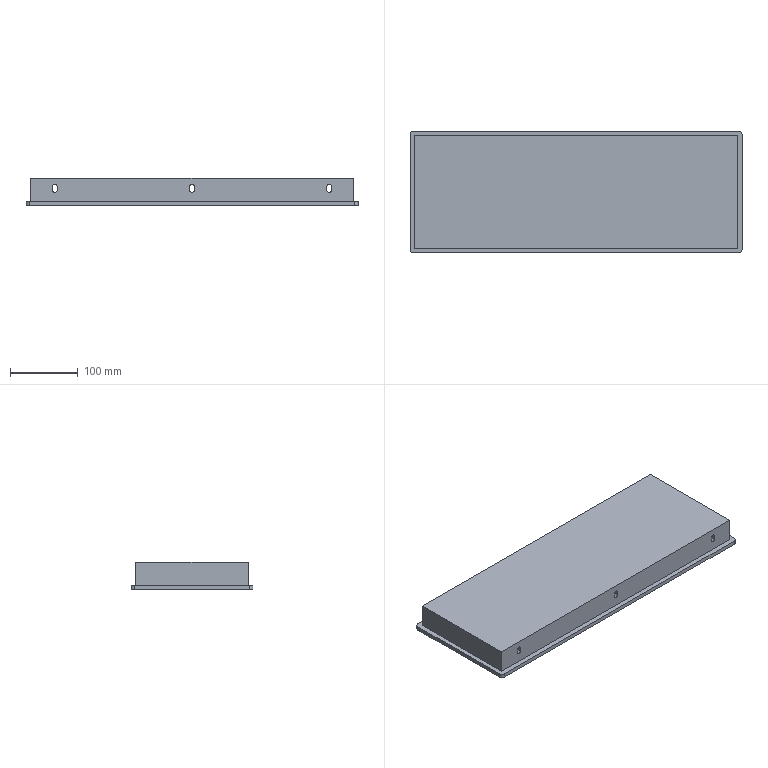Part | 1 solid | 30 faces | box 490 x 180 x 41 mm | volume 3258036 mm3 | plane 17 | cylinder 13 | commonest cylinder face diameters 7 x9 10 x4
STEP:
#1=CARTESIAN_POINT('',(-202.5,-83.,32.));
#2=VERTEX_POINT('',#1);
#3=CARTESIAN_POINT('',(-199.,-83.,28.5));
#4=VERTEX_POINT('',#3);
#5=CARTESIAN_POINT('',(-202.5,-83.,28.5));
#6=DIRECTION('',(0.,1.,0.));
#7=DIRECTION('',(0.,0.,1.));
#8=AXIS2_PLACEMENT_3D('',#5,#6,#7);
#9=CIRCLE('',#8,3.5);
#10=EDGE_CURVE('',#2,#4,#9,.T.);
#11=ORIENTED_EDGE('',*,*,#10,.F.);
#12=CARTESIAN_POINT('',(-202.5,83.,32.));
#13=VERTEX_POINT('',#12);
#14=CARTESIAN_POINT('',(-202.5,-90.,32.));
#15=DIRECTION('',(0.,1.,0.));
#16=VECTOR('',#15,1000.);
#17=LINE('',#14,#16);
#18=EDGE_CURVE('',#2,#13,#17,.T.);
#19=ORIENTED_EDGE('',*,*,#18,.T.);
#20=CARTESIAN_POINT('',(-199.,83.,28.5));
#21=VERTEX_POINT('',#20);
#22=CARTESIAN_POINT('',(-202.5,83.,28.5));
#23=DIRECTION('',(0.,-1.,0.));
#24=DIRECTION('',(0.,0.,-1.));
#25=AXIS2_PLACEMENT_3D('',#22,#23,#24);
#26=CIRCLE('',#25,3.5);
#27=EDGE_CURVE('',#21,#13,#26,.T.);
#28=ORIENTED_EDGE('',*,*,#27,.F.);
#29=CARTESIAN_POINT('',(-199.,-90.,28.5));
#30=DIRECTION('',(0.,1.,0.));
#31=VECTOR('',#30,1000.);
#32=LINE('',#29,#31);
#33=EDGE_CURVE('',#4,#21,#32,.T.);
#34=ORIENTED_EDGE('',*,*,#33,.F.);
#35=EDGE_LOOP('',(#11,#19,#28,#34));
#36=FACE_OUTER_BOUND('',#35,.T.);
#37=CARTESIAN_POINT('',(-202.5,-90.,28.5));
#38=DIRECTION('',(0.,1.,0.));
#39=DIRECTION('',(0.,0.,1.));
#40=AXIS2_PLACEMENT_3D('',#37,#38,#39);
#41=CYLINDRICAL_SURFACE('',#40,3.5);
#42=ADVANCED_FACE('',(#36),#41,.F.);
#43=CARTESIAN_POINT('',(0.,-83.,32.));
#44=VERTEX_POINT('',#43);
#45=CARTESIAN_POINT('',(3.5,-83.,28.5));
#46=VERTEX_POINT('',#45);
#47=CARTESIAN_POINT('',(0.,-83.,28.5));
#48=DIRECTION('',(0.,1.,0.));
#49=DIRECTION('',(0.,0.,1.));
#50=AXIS2_PLACEMENT_3D('',#47,#48,#49);
#51=CIRCLE('',#50,3.5);
#52=EDGE_CURVE('',#44,#46,#51,.T.);
#53=ORIENTED_EDGE('',*,*,#52,.F.);
#54=CARTESIAN_POINT('',(0.,83.,32.));
#55=VERTEX_POINT('',#54);
#56=CARTESIAN_POINT('',(0.,-90.,32.));
#57=DIRECTION('',(0.,1.,0.));
#58=VECTOR('',#57,1000.);
#59=LINE('',#56,#58);
#60=EDGE_CURVE('',#44,#55,#59,.T.);
#61=ORIENTED_EDGE('',*,*,#60,.T.);
#62=CARTESIAN_POINT('',(3.5,83.,28.5));
#63=VERTEX_POINT('',#62);
#64=CARTESIAN_POINT('',(0.,83.,28.5));
#65=DIRECTION('',(0.,-1.,0.));
#66=DIRECTION('',(0.,0.,-1.));
#67=AXIS2_PLACEMENT_3D('',#64,#65,#66);
#68=CIRCLE('',#67,3.5);
#69=EDGE_CURVE('',#63,#55,#68,.T.);
#70=ORIENTED_EDGE('',*,*,#69,.F.);
#71=CARTESIAN_POINT('',(3.5,-90.,28.5));
#72=DIRECTION('',(0.,1.,0.));
#73=VECTOR('',#72,1000.);
#74=LINE('',#71,#73);
#75=EDGE_CURVE('',#46,#63,#74,.T.);
#76=ORIENTED_EDGE('',*,*,#75,.F.);
#77=EDGE_LOOP('',(#53,#61,#70,#76));
#78=FACE_OUTER_BOUND('',#77,.T.);
#79=CARTESIAN_POINT('',(0.,-90.,28.5));
#80=DIRECTION('',(0.,1.,0.));
#81=DIRECTION('',(0.,0.,1.));
#82=AXIS2_PLACEMENT_3D('',#79,#80,#81);
#83=CYLINDRICAL_SURFACE('',#82,3.5);
#84=ADVANCED_FACE('',(#78),#83,.F.);
#85=CARTESIAN_POINT('',(202.5,-83.,32.));
#86=VERTEX_POINT('',#85);
#87=CARTESIAN_POINT('',(206.,-83.,28.5));
#88=VERTEX_POINT('',#87);
#89=CARTESIAN_POINT('',(202.5,-83.,28.5));
#90=DIRECTION('',(0.,1.,0.));
#91=DIRECTION('',(0.,0.,1.));
#92=AXIS2_PLACEMENT_3D('',#89,#90,#91);
#93=CIRCLE('',#92,3.5);
#94=EDGE_CURVE('',#86,#88,#93,.T.);
#95=ORIENTED_EDGE('',*,*,#94,.F.);
#96=CARTESIAN_POINT('',(202.5,83.,32.));
#97=VERTEX_POINT('',#96);
#98=CARTESIAN_POINT('',(202.5,-90.,32.));
#99=DIRECTION('',(0.,1.,0.));
#100=VECTOR('',#99,1000.);
#101=LINE('',#98,#100);
#102=EDGE_CURVE('',#86,#97,#101,.T.);
#103=ORIENTED_EDGE('',*,*,#102,.T.);
#104=CARTESIAN_POINT('',(206.,83.,28.5));
#105=VERTEX_POINT('',#104);
#106=CARTESIAN_POINT('',(202.5,83.,28.5));
#107=DIRECTION('',(0.,-1.,0.));
#108=DIRECTION('',(0.,0.,-1.));
#109=AXIS2_PLACEMENT_3D('',#106,#107,#108);
#110=CIRCLE('',#109,3.5);
#111=EDGE_CURVE('',#105,#97,#110,.T.);
#112=ORIENTED_EDGE('',*,*,#111,.F.);
#113=CARTESIAN_POINT('',(206.,-90.,28.5));
#114=DIRECTION('',(0.,1.,0.));
#115=VECTOR('',#114,1000.);
#116=LINE('',#113,#115);
#117=EDGE_CURVE('',#88,#105,#116,.T.);
#118=ORIENTED_EDGE('',*,*,#117,.F.);
#119=EDGE_LOOP('',(#95,#103,#112,#118));
#120=FACE_OUTER_BOUND('',#119,.T.);
#121=CARTESIAN_POINT('',(202.5,-90.,28.5));
#122=DIRECTION('',(0.,1.,0.));
#123=DIRECTION('',(0.,0.,1.));
#124=AXIS2_PLACEMENT_3D('',#121,#122,#123);
#125=CYLINDRICAL_SURFACE('',#124,3.5);
#126=ADVANCED_FACE('',(#120),#125,.F.);
#127=CARTESIAN_POINT('',(245.,-85.,0.));
#128=VERTEX_POINT('',#127);
#129=CARTESIAN_POINT('',(245.,85.,0.));
#130=VERTEX_POINT('',#129);
#131=CARTESIAN_POINT('',(245.,90.,0.));
#132=DIRECTION('',(0.,1.,0.));
#133=VECTOR('',#132,1000.);
#134=LINE('',#131,#133);
#135=EDGE_CURVE('',#128,#130,#134,.T.);
#136=ORIENTED_EDGE('',*,*,#135,.T.);
#137=CARTESIAN_POINT('',(245.,85.,6.));
#138=VERTEX_POINT('',#137);
#139=CARTESIAN_POINT('',(245.,85.,6.));
#140=DIRECTION('',(0.,0.,1.));
#141=VECTOR('',#140,1000.);
#142=LINE('',#139,#141);
#143=EDGE_CURVE('',#130,#138,#142,.T.);
#144=ORIENTED_EDGE('',*,*,#143,.T.);
#145=CARTESIAN_POINT('',(245.,-85.,6.));
#146=VERTEX_POINT('',#145);
#147=CARTESIAN_POINT('',(245.,90.,6.));
#148=DIRECTION('',(0.,1.,0.));
#149=VECTOR('',#148,1000.);
#150=LINE('',#147,#149);
#151=EDGE_CURVE('',#146,#138,#150,.T.);
#152=ORIENTED_EDGE('',*,*,#151,.F.);
#153=CARTESIAN_POINT('',(245.,-85.,6.));
#154=DIRECTION('',(0.,0.,-1.));
#155=VECTOR('',#154,1000.);
#156=LINE('',#153,#155);
#157=EDGE_CURVE('',#146,#128,#156,.T.);
#158=ORIENTED_EDGE('',*,*,#157,.T.);
#159=EDGE_LOOP('',(#136,#144,#152,#158));
#160=FACE_OUTER_BOUND('',#159,.T.);
#161=CARTESIAN_POINT('',(245.,90.,6.));
#162=DIRECTION('',(-1.,0.,0.));
#163=DIRECTION('',(0.,0.,1.));
#164=AXIS2_PLACEMENT_3D('',#161,#162,#163);
#165=PLANE('',#164);
#166=ADVANCED_FACE('',(#160),#165,.F.);
#167=CARTESIAN_POINT('',(240.,90.,6.));
#168=VERTEX_POINT('',#167);
#169=CARTESIAN_POINT('',(-240.,90.,6.));
#170=VERTEX_POINT('',#169);
#171=CARTESIAN_POINT('',(-245.,90.,6.));
#172=DIRECTION('',(-1.,0.,0.));
#173=VECTOR('',#172,1000.);
#174=LINE('',#171,#173);
#175=EDGE_CURVE('',#168,#170,#174,.T.);
#176=ORIENTED_EDGE('',*,*,#175,.F.);
#177=CARTESIAN_POINT('',(240.,90.,0.));
#178=VERTEX_POINT('',#177);
#179=CARTESIAN_POINT('',(240.,90.,6.));
#180=DIRECTION('',(0.,0.,-1.));
#181=VECTOR('',#180,1000.);
#182=LINE('',#179,#181);
#183=EDGE_CURVE('',#168,#178,#182,.T.);
#184=ORIENTED_EDGE('',*,*,#183,.T.);
#185=CARTESIAN_POINT('',(-240.,90.,0.));
#186=VERTEX_POINT('',#185);
#187=CARTESIAN_POINT('',(-245.,90.,0.));
#188=DIRECTION('',(-1.,0.,0.));
#189=VECTOR('',#188,1000.);
#190=LINE('',#187,#189);
#191=EDGE_CURVE('',#178,#186,#190,.T.);
#192=ORIENTED_EDGE('',*,*,#191,.T.);
#193=CARTESIAN_POINT('',(-240.,90.,6.));
#194=DIRECTION('',(0.,0.,1.));
#195=VECTOR('',#194,1000.);
#196=LINE('',#193,#195);
#197=EDGE_CURVE('',#186,#170,#196,.T.);
#198=ORIENTED_EDGE('',*,*,#197,.T.);
#199=EDGE_LOOP('',(#176,#184,#192,#198));
#200=FACE_OUTER_BOUND('',#199,.T.);
#201=CARTESIAN_POINT('',(-245.,90.,6.));
#202=DIRECTION('',(0.,-1.,0.));
#203=DIRECTION('',(0.,0.,-1.));
#204=AXIS2_PLACEMENT_3D('',#201,#202,#203);
#205=PLANE('',#204);
#206=ADVANCED_FACE('',(#200),#205,.F.);
#207=CARTESIAN_POINT('',(-245.,85.,0.));
#208=VERTEX_POINT('',#207);
#209=CARTESIAN_POINT('',(-245.,-85.,0.));
#210=VERTEX_POINT('',#209);
#211=CARTESIAN_POINT('',(-245.,90.,0.));
#212=DIRECTION('',(0.,-1.,0.));
#213=VECTOR('',#212,1000.);
#214=LINE('',#211,#213);
#215=EDGE_CURVE('',#208,#210,#214,.T.);
#216=ORIENTED_EDGE('',*,*,#215,.T.);
#217=CARTESIAN_POINT('',(-245.,-85.,6.));
#218=VERTEX_POINT('',#217);
#219=CARTESIAN_POINT('',(-245.,-85.,6.));
#220=DIRECTION('',(0.,0.,1.));
#221=VECTOR('',#220,1000.);
#222=LINE('',#219,#221);
#223=EDGE_CURVE('',#210,#218,#222,.T.);
#224=ORIENTED_EDGE('',*,*,#223,.T.);
#225=CARTESIAN_POINT('',(-245.,85.,6.));
#226=VERTEX_POINT('',#225);
#227=CARTESIAN_POINT('',(-245.,90.,6.));
#228=DIRECTION('',(0.,-1.,0.));
#229=VECTOR('',#228,1000.);
#230=LINE('',#227,#229);
#231=EDGE_CURVE('',#226,#218,#230,.T.);
#232=ORIENTED_EDGE('',*,*,#231,.F.);
#233=CARTESIAN_POINT('',(-245.,85.,6.));
#234=DIRECTION('',(0.,0.,-1.));
#235=VECTOR('',#234,1000.);
#236=LINE('',#233,#235);
#237=EDGE_CURVE('',#226,#208,#236,.T.);
#238=ORIENTED_EDGE('',*,*,#237,.T.);
#239=EDGE_LOOP('',(#216,#224,#232,#238));
#240=FACE_OUTER_BOUND('',#239,.T.);
#241=CARTESIAN_POINT('',(-245.,90.,6.));
#242=DIRECTION('',(1.,0.,0.));
#243=DIRECTION('',(0.,0.,-1.));
#244=AXIS2_PLACEMENT_3D('',#241,#242,#243);
#245=PLANE('',#244);
#246=ADVANCED_FACE('',(#240),#245,.F.);
#247=CARTESIAN_POINT('',(-240.,-90.,0.));
#248=VERTEX_POINT('',#247);
#249=CARTESIAN_POINT('',(240.,-90.,0.));
#250=VERTEX_POINT('',#249);
#251=CARTESIAN_POINT('',(-245.,-90.,0.));
#252=DIRECTION('',(1.,0.,0.));
#253=VECTOR('',#252,1000.);
#254=LINE('',#251,#253);
#255=EDGE_CURVE('',#248,#250,#254,.T.);
#256=ORIENTED_EDGE('',*,*,#255,.T.);
#257=CARTESIAN_POINT('',(240.,-90.,6.));
#258=VERTEX_POINT('',#257);
#259=CARTESIAN_POINT('',(240.,-90.,6.));
#260=DIRECTION('',(0.,0.,1.));
#261=VECTOR('',#260,1000.);
#262=LINE('',#259,#261);
#263=EDGE_CURVE('',#250,#258,#262,.T.);
#264=ORIENTED_EDGE('',*,*,#263,.T.);
#265=CARTESIAN_POINT('',(-240.,-90.,6.));
#266=VERTEX_POINT('',#265);
#267=CARTESIAN_POINT('',(-245.,-90.,6.));
#268=DIRECTION('',(1.,0.,0.));
#269=VECTOR('',#268,1000.);
#270=LINE('',#267,#269);
#271=EDGE_CURVE('',#266,#258,#270,.T.);
#272=ORIENTED_EDGE('',*,*,#271,.F.);
#273=CARTESIAN_POINT('',(-240.,-90.,6.));
#274=DIRECTION('',(0.,0.,-1.));
#275=VECTOR('',#274,1000.);
#276=LINE('',#273,#275);
#277=EDGE_CURVE('',#266,#248,#276,.T.);
#278=ORIENTED_EDGE('',*,*,#277,.T.);
#279=EDGE_LOOP('',(#256,#264,#272,#278));
#280=FACE_OUTER_BOUND('',#279,.T.);
#281=CARTESIAN_POINT('',(-245.,-90.,6.));
#282=DIRECTION('',(0.,1.,0.));
#283=DIRECTION('',(0.,0.,1.));
#284=AXIS2_PLACEMENT_3D('',#281,#282,#283);
#285=PLANE('',#284);
#286=ADVANCED_FACE('',(#280),#285,.F.);
#287=CARTESIAN_POINT('',(238.,-83.,6.));
#288=VERTEX_POINT('',#287);
#289=CARTESIAN_POINT('',(238.,83.,6.));
#290=VERTEX_POINT('',#289);
#291=CARTESIAN_POINT('',(238.,83.,6.));
#292=DIRECTION('',(0.,1.,0.));
#293=VECTOR('',#292,1000.);
#294=LINE('',#291,#293);
#295=EDGE_CURVE('',#288,#290,#294,.T.);
#296=ORIENTED_EDGE('',*,*,#295,.F.);
#297=CARTESIAN_POINT('',(-238.,-83.,6.));
#298=VERTEX_POINT('',#297);
#299=CARTESIAN_POINT('',(-238.,-83.,6.));
#300=DIRECTION('',(1.,0.,0.));
#301=VECTOR('',#300,1000.);
#302=LINE('',#299,#301);
#303=EDGE_CURVE('',#298,#288,#302,.T.);
#304=ORIENTED_EDGE('',*,*,#303,.F.);
#305=CARTESIAN_POINT('',(-238.,83.,6.));
#306=VERTEX_POINT('',#305);
#307=CARTESIAN_POINT('',(-238.,83.,6.));
#308=DIRECTION('',(0.,-1.,0.));
#309=VECTOR('',#308,1000.);
#310=LINE('',#307,#309);
#311=EDGE_CURVE('',#306,#298,#310,.T.);
#312=ORIENTED_EDGE('',*,*,#311,.F.);
#313=CARTESIAN_POINT('',(-238.,83.,6.));
#314=DIRECTION('',(-1.,0.,0.));
#315=VECTOR('',#314,1000.);
#316=LINE('',#313,#315);
#317=EDGE_CURVE('',#290,#306,#316,.T.);
#318=ORIENTED_EDGE('',*,*,#317,.F.);
#319=EDGE_LOOP('',(#296,#304,#312,#318));
#320=FACE_BOUND('',#319,.T.);
#321=ORIENTED_EDGE('',*,*,#151,.T.);
#322=CARTESIAN_POINT('',(240.,85.,6.));
#323=DIRECTION('',(0.,0.,1.));
#324=DIRECTION('',(1.,0.,0.));
#325=AXIS2_PLACEMENT_3D('',#322,#323,#324);
#326=CIRCLE('',#325,5.);
#327=EDGE_CURVE('',#138,#168,#326,.T.);
#328=ORIENTED_EDGE('',*,*,#327,.T.);
#329=ORIENTED_EDGE('',*,*,#175,.T.);
#330=CARTESIAN_POINT('',(-240.,85.,6.));
#331=DIRECTION('',(0.,0.,1.));
#332=DIRECTION('',(1.,0.,0.));
#333=AXIS2_PLACEMENT_3D('',#330,#331,#332);
#334=CIRCLE('',#333,5.);
#335=EDGE_CURVE('',#170,#226,#334,.T.);
#336=ORIENTED_EDGE('',*,*,#335,.T.);
#337=ORIENTED_EDGE('',*,*,#231,.T.);
#338=CARTESIAN_POINT('',(-240.,-85.,6.));
#339=DIRECTION('',(0.,0.,1.));
#340=DIRECTION('',(1.,0.,0.));
#341=AXIS2_PLACEMENT_3D('',#338,#339,#340);
#342=CIRCLE('',#341,5.);
#343=EDGE_CURVE('',#218,#266,#342,.T.);
#344=ORIENTED_EDGE('',*,*,#343,.T.);
#345=ORIENTED_EDGE('',*,*,#271,.T.);
#346=CARTESIAN_POINT('',(240.,-85.,6.));
#347=DIRECTION('',(0.,0.,1.));
#348=DIRECTION('',(1.,0.,0.));
#349=AXIS2_PLACEMENT_3D('',#346,#347,#348);
#350=CIRCLE('',#349,5.);
#351=EDGE_CURVE('',#258,#146,#350,.T.);
#352=ORIENTED_EDGE('',*,*,#351,.T.);
#353=EDGE_LOOP('',(#321,#328,#329,#336,#337,#344,#345,#352));
#354=FACE_OUTER_BOUND('',#353,.T.);
#355=CARTESIAN_POINT('',(0.,0.,6.));
#356=DIRECTION('',(0.,0.,1.));
#357=DIRECTION('',(1.,0.,0.));
#358=AXIS2_PLACEMENT_3D('',#355,#356,#357);
#359=PLANE('',#358);
#360=ADVANCED_FACE('',(#320,#354),#359,.T.);
#361=ORIENTED_EDGE('',*,*,#191,.F.);
#362=CARTESIAN_POINT('',(240.,85.,0.));
#363=DIRECTION('',(0.,0.,-1.));
#364=DIRECTION('',(1.,0.,0.));
#365=AXIS2_PLACEMENT_3D('',#362,#363,#364);
#366=CIRCLE('',#365,5.);
#367=EDGE_CURVE('',#178,#130,#366,.T.);
#368=ORIENTED_EDGE('',*,*,#367,.T.);
#369=ORIENTED_EDGE('',*,*,#135,.F.);
#370=CARTESIAN_POINT('',(240.,-85.,0.));
#371=DIRECTION('',(0.,0.,-1.));
#372=DIRECTION('',(1.,0.,0.));
#373=AXIS2_PLACEMENT_3D('',#370,#371,#372);
#374=CIRCLE('',#373,5.);
#375=EDGE_CURVE('',#128,#250,#374,.T.);
#376=ORIENTED_EDGE('',*,*,#375,.T.);
#377=ORIENTED_EDGE('',*,*,#255,.F.);
#378=CARTESIAN_POINT('',(-240.,-85.,0.));
#379=DIRECTION('',(0.,0.,-1.));
#380=DIRECTION('',(1.,0.,0.));
#381=AXIS2_PLACEMENT_3D('',#378,#379,#380);
#382=CIRCLE('',#381,5.);
#383=EDGE_CURVE('',#248,#210,#382,.T.);
#384=ORIENTED_EDGE('',*,*,#383,.T.);
#385=ORIENTED_EDGE('',*,*,#215,.F.);
#386=CARTESIAN_POINT('',(-240.,85.,0.));
#387=DIRECTION('',(0.,0.,-1.));
#388=DIRECTION('',(1.,0.,0.));
#389=AXIS2_PLACEMENT_3D('',#386,#387,#388);
#390=CIRCLE('',#389,5.);
#391=EDGE_CURVE('',#208,#186,#390,.T.);
#392=ORIENTED_EDGE('',*,*,#391,.T.);
#393=EDGE_LOOP('',(#361,#368,#369,#376,#377,#384,#385,#392));
#394=FACE_OUTER_BOUND('',#393,.T.);
#395=CARTESIAN_POINT('',(0.,0.,0.));
#396=DIRECTION('',(0.,0.,1.));
#397=DIRECTION('',(1.,0.,0.));
#398=AXIS2_PLACEMENT_3D('',#395,#396,#397);
#399=PLANE('',#398);
#400=ADVANCED_FACE('',(#394),#399,.F.);
#401=ORIENTED_EDGE('',*,*,#295,.T.);
#402=CARTESIAN_POINT('',(238.,83.,41.));
#403=VERTEX_POINT('',#402);
#404=CARTESIAN_POINT('',(238.,83.,41.));
#405=DIRECTION('',(0.,0.,-1.));
#406=VECTOR('',#405,1000.);
#407=LINE('',#404,#406);
#408=EDGE_CURVE('',#403,#290,#407,.T.);
#409=ORIENTED_EDGE('',*,*,#408,.F.);
#410=CARTESIAN_POINT('',(238.,-83.,41.));
#411=VERTEX_POINT('',#410);
#412=CARTESIAN_POINT('',(238.,83.,41.));
#413=DIRECTION('',(0.,1.,0.));
#414=VECTOR('',#413,1000.);
#415=LINE('',#412,#414);
#416=EDGE_CURVE('',#411,#403,#415,.T.);
#417=ORIENTED_EDGE('',*,*,#416,.F.);
#418=CARTESIAN_POINT('',(238.,-83.,41.));
#419=DIRECTION('',(0.,0.,-1.));
#420=VECTOR('',#419,1000.);
#421=LINE('',#418,#420);
#422=EDGE_CURVE('',#411,#288,#421,.T.);
#423=ORIENTED_EDGE('',*,*,#422,.T.);
#424=EDGE_LOOP('',(#401,#409,#417,#423));
#425=FACE_OUTER_BOUND('',#424,.T.);
#426=CARTESIAN_POINT('',(238.,83.,41.));
#427=DIRECTION('',(-1.,0.,0.));
#428=DIRECTION('',(0.,-1.,0.));
#429=AXIS2_PLACEMENT_3D('',#426,#427,#428);
#430=PLANE('',#429);
#431=ADVANCED_FACE('',(#425),#430,.F.);
#432=CARTESIAN_POINT('',(-206.,83.,28.5));
#433=VERTEX_POINT('',#432);
#434=CARTESIAN_POINT('',(-206.,83.,23.5));
#435=VERTEX_POINT('',#434);
#436=CARTESIAN_POINT('',(-206.,83.,41.));
#437=DIRECTION('',(0.,0.,-1.));
#438=VECTOR('',#437,1000.);
#439=LINE('',#436,#438);
#440=EDGE_CURVE('',#433,#435,#439,.T.);
#441=ORIENTED_EDGE('',*,*,#440,.T.);
#442=CARTESIAN_POINT('',(-199.,83.,23.5));
#443=VERTEX_POINT('',#442);
#444=CARTESIAN_POINT('',(-202.5,83.,23.5));
#445=DIRECTION('',(0.,-1.,0.));
#446=DIRECTION('',(0.,0.,-1.));
#447=AXIS2_PLACEMENT_3D('',#444,#445,#446);
#448=CIRCLE('',#447,3.5);
#449=EDGE_CURVE('',#435,#443,#448,.T.);
#450=ORIENTED_EDGE('',*,*,#449,.T.);
#451=CARTESIAN_POINT('',(-199.,83.,41.));
#452=DIRECTION('',(0.,0.,1.));
#453=VECTOR('',#452,1000.);
#454=LINE('',#451,#453);
#455=EDGE_CURVE('',#443,#21,#454,.T.);
#456=ORIENTED_EDGE('',*,*,#455,.T.);
#457=ORIENTED_EDGE('',*,*,#27,.T.);
#458=CARTESIAN_POINT('',(-202.5,83.,28.5));
#459=DIRECTION('',(0.,-1.,0.));
#460=DIRECTION('',(0.,0.,-1.));
#461=AXIS2_PLACEMENT_3D('',#458,#459,#460);
#462=CIRCLE('',#461,3.5);
#463=EDGE_CURVE('',#13,#433,#462,.T.);
#464=ORIENTED_EDGE('',*,*,#463,.T.);
#465=EDGE_LOOP('',(#441,#450,#456,#457,#464));
#466=FACE_BOUND('',#465,.T.);
#467=CARTESIAN_POINT('',(-3.5,83.,28.5));
#468=VERTEX_POINT('',#467);
#469=CARTESIAN_POINT('',(-3.5,83.,23.5));
#470=VERTEX_POINT('',#469);
#471=CARTESIAN_POINT('',(-3.5,83.,41.));
#472=DIRECTION('',(0.,0.,-1.));
#473=VECTOR('',#472,1000.);
#474=LINE('',#471,#473);
#475=EDGE_CURVE('',#468,#470,#474,.T.);
#476=ORIENTED_EDGE('',*,*,#475,.T.);
#477=CARTESIAN_POINT('',(3.5,83.,23.5));
#478=VERTEX_POINT('',#477);
#479=CARTESIAN_POINT('',(0.,83.,23.5));
#480=DIRECTION('',(0.,-1.,0.));
#481=DIRECTION('',(0.,0.,-1.));
#482=AXIS2_PLACEMENT_3D('',#479,#480,#481);
#483=CIRCLE('',#482,3.5);
#484=EDGE_CURVE('',#470,#478,#483,.T.);
#485=ORIENTED_EDGE('',*,*,#484,.T.);
#486=CARTESIAN_POINT('',(3.5,83.,41.));
#487=DIRECTION('',(0.,0.,1.));
#488=VECTOR('',#487,1000.);
#489=LINE('',#486,#488);
#490=EDGE_CURVE('',#478,#63,#489,.T.);
#491=ORIENTED_EDGE('',*,*,#490,.T.);
#492=ORIENTED_EDGE('',*,*,#69,.T.);
#493=CARTESIAN_POINT('',(0.,83.,28.5));
#494=DIRECTION('',(0.,-1.,0.));
#495=DIRECTION('',(0.,0.,-1.));
#496=AXIS2_PLACEMENT_3D('',#493,#494,#495);
#497=CIRCLE('',#496,3.5);
#498=EDGE_CURVE('',#55,#468,#497,.T.);
#499=ORIENTED_EDGE('',*,*,#498,.T.);
#500=EDGE_LOOP('',(#476,#485,#491,#492,#499));
#501=FACE_BOUND('',#500,.T.);
#502=CARTESIAN_POINT('',(199.,83.,28.5));
#503=VERTEX_POINT('',#502);
#504=CARTESIAN_POINT('',(199.,83.,23.5));
#505=VERTEX_POINT('',#504);
#506=CARTESIAN_POINT('',(199.,83.,41.));
#507=DIRECTION('',(0.,0.,-1.));
#508=VECTOR('',#507,1000.);
#509=LINE('',#506,#508);
#510=EDGE_CURVE('',#503,#505,#509,.T.);
#511=ORIENTED_EDGE('',*,*,#510,.T.);
#512=CARTESIAN_POINT('',(206.,83.,23.5));
#513=VERTEX_POINT('',#512);
#514=CARTESIAN_POINT('',(202.5,83.,23.5));
#515=DIRECTION('',(0.,-1.,0.));
#516=DIRECTION('',(0.,0.,-1.));
#517=AXIS2_PLACEMENT_3D('',#514,#515,#516);
#518=CIRCLE('',#517,3.5);
#519=EDGE_CURVE('',#505,#513,#518,.T.);
#520=ORIENTED_EDGE('',*,*,#519,.T.);
#521=CARTESIAN_POINT('',(206.,83.,41.));
#522=DIRECTION('',(0.,0.,1.));
#523=VECTOR('',#522,1000.);
#524=LINE('',#521,#523);
#525=EDGE_CURVE('',#513,#105,#524,.T.);
#526=ORIENTED_EDGE('',*,*,#525,.T.);
#527=ORIENTED_EDGE('',*,*,#111,.T.);
#528=CARTESIAN_POINT('',(202.5,83.,28.5));
#529=DIRECTION('',(0.,-1.,0.));
#530=DIRECTION('',(0.,0.,-1.));
#531=AXIS2_PLACEMENT_3D('',#528,#529,#530);
#532=CIRCLE('',#531,3.5);
#533=EDGE_CURVE('',#97,#503,#532,.T.);
#534=ORIENTED_EDGE('',*,*,#533,.T.);
#535=EDGE_LOOP('',(#511,#520,#526,#527,#534));
#536=FACE_BOUND('',#535,.T.);
#537=ORIENTED_EDGE('',*,*,#317,.T.);
#538=CARTESIAN_POINT('',(-238.,83.,41.));
#539=VERTEX_POINT('',#538);
#540=CARTESIAN_POINT('',(-238.,83.,41.));
#541=DIRECTION('',(0.,0.,-1.));
#542=VECTOR('',#541,1000.);
#543=LINE('',#540,#542);
#544=EDGE_CURVE('',#539,#306,#543,.T.);
#545=ORIENTED_EDGE('',*,*,#544,.F.);
#546=CARTESIAN_POINT('',(-238.,83.,41.));
#547=DIRECTION('',(-1.,0.,0.));
#548=VECTOR('',#547,1000.);
#549=LINE('',#546,#548);
#550=EDGE_CURVE('',#403,#539,#549,.T.);
#551=ORIENTED_EDGE('',*,*,#550,.F.);
#552=ORIENTED_EDGE('',*,*,#408,.T.);
#553=EDGE_LOOP('',(#537,#545,#551,#552));
#554=FACE_OUTER_BOUND('',#553,.T.);
#555=CARTESIAN_POINT('',(-238.,83.,41.));
#556=DIRECTION('',(0.,-1.,0.));
#557=DIRECTION('',(0.,0.,-1.));
#558=AXIS2_PLACEMENT_3D('',#555,#556,#557);
#559=PLANE('',#558);
#560=ADVANCED_FACE('',(#466,#501,#536,#554),#559,.F.);
#561=ORIENTED_EDGE('',*,*,#311,.T.);
#562=CARTESIAN_POINT('',(-238.,-83.,41.));
#563=VERTEX_POINT('',#562);
#564=CARTESIAN_POINT('',(-238.,-83.,41.));
#565=DIRECTION('',(0.,0.,-1.));
#566=VECTOR('',#565,1000.);
#567=LINE('',#564,#566);
#568=EDGE_CURVE('',#563,#298,#567,.T.);
#569=ORIENTED_EDGE('',*,*,#568,.F.);
#570=CARTESIAN_POINT('',(-238.,83.,41.));
#571=DIRECTION('',(0.,-1.,0.));
#572=VECTOR('',#571,1000.);
#573=LINE('',#570,#572);
#574=EDGE_CURVE('',#539,#563,#573,.T.);
#575=ORIENTED_EDGE('',*,*,#574,.F.);
#576=ORIENTED_EDGE('',*,*,#544,.T.);
#577=EDGE_LOOP('',(#561,#569,#575,#576));
#578=FACE_OUTER_BOUND('',#577,.T.);
#579=CARTESIAN_POINT('',(-238.,83.,41.));
#580=DIRECTION('',(1.,0.,0.));
#581=DIRECTION('',(0.,1.,0.));
#582=AXIS2_PLACEMENT_3D('',#579,#580,#581);
#583=PLANE('',#582);
#584=ADVANCED_FACE('',(#578),#583,.F.);
#585=CARTESIAN_POINT('',(-199.,-83.,23.5));
#586=VERTEX_POINT('',#585);
#587=CARTESIAN_POINT('',(-199.,-83.,41.));
#588=DIRECTION('',(0.,0.,-1.));
#589=VECTOR('',#588,1000.);
#590=LINE('',#587,#589);
#591=EDGE_CURVE('',#4,#586,#590,.T.);
#592=ORIENTED_EDGE('',*,*,#591,.T.);
#593=CARTESIAN_POINT('',(-206.,-83.,23.5));
#594=VERTEX_POINT('',#593);
#595=CARTESIAN_POINT('',(-202.5,-83.,23.5));
#596=DIRECTION('',(0.,1.,0.));
#597=DIRECTION('',(0.,0.,1.));
#598=AXIS2_PLACEMENT_3D('',#595,#596,#597);
#599=CIRCLE('',#598,3.5);
#600=EDGE_CURVE('',#586,#594,#599,.T.);
#601=ORIENTED_EDGE('',*,*,#600,.T.);
#602=CARTESIAN_POINT('',(-206.,-83.,28.5));
#603=VERTEX_POINT('',#602);
#604=CARTESIAN_POINT('',(-206.,-83.,41.));
#605=DIRECTION('',(0.,0.,1.));
#606=VECTOR('',#605,1000.);
#607=LINE('',#604,#606);
#608=EDGE_CURVE('',#594,#603,#607,.T.);
#609=ORIENTED_EDGE('',*,*,#608,.T.);
#610=CARTESIAN_POINT('',(-202.5,-83.,28.5));
#611=DIRECTION('',(0.,1.,0.));
#612=DIRECTION('',(0.,0.,1.));
#613=AXIS2_PLACEMENT_3D('',#610,#611,#612);
#614=CIRCLE('',#613,3.5);
#615=EDGE_CURVE('',#603,#2,#614,.T.);
#616=ORIENTED_EDGE('',*,*,#615,.T.);
#617=ORIENTED_EDGE('',*,*,#10,.T.);
#618=EDGE_LOOP('',(#592,#601,#609,#616,#617));
#619=FACE_BOUND('',#618,.T.);
#620=CARTESIAN_POINT('',(3.5,-83.,23.5));
#621=VERTEX_POINT('',#620);
#622=CARTESIAN_POINT('',(3.5,-83.,41.));
#623=DIRECTION('',(0.,0.,-1.));
#624=VECTOR('',#623,1000.);
#625=LINE('',#622,#624);
#626=EDGE_CURVE('',#46,#621,#625,.T.);
#627=ORIENTED_EDGE('',*,*,#626,.T.);
#628=CARTESIAN_POINT('',(-3.5,-83.,23.5));
#629=VERTEX_POINT('',#628);
#630=CARTESIAN_POINT('',(0.,-83.,23.5));
#631=DIRECTION('',(0.,1.,0.));
#632=DIRECTION('',(0.,0.,1.));
#633=AXIS2_PLACEMENT_3D('',#630,#631,#632);
#634=CIRCLE('',#633,3.5);
#635=EDGE_CURVE('',#621,#629,#634,.T.);
#636=ORIENTED_EDGE('',*,*,#635,.T.);
#637=CARTESIAN_POINT('',(-3.5,-83.,28.5));
#638=VERTEX_POINT('',#637);
#639=CARTESIAN_POINT('',(-3.5,-83.,41.));
#640=DIRECTION('',(0.,0.,1.));
#641=VECTOR('',#640,1000.);
#642=LINE('',#639,#641);
#643=EDGE_CURVE('',#629,#638,#642,.T.);
#644=ORIENTED_EDGE('',*,*,#643,.T.);
#645=CARTESIAN_POINT('',(0.,-83.,28.5));
#646=DIRECTION('',(0.,1.,0.));
#647=DIRECTION('',(0.,0.,1.));
#648=AXIS2_PLACEMENT_3D('',#645,#646,#647);
#649=CIRCLE('',#648,3.5);
#650=EDGE_CURVE('',#638,#44,#649,.T.);
#651=ORIENTED_EDGE('',*,*,#650,.T.);
#652=ORIENTED_EDGE('',*,*,#52,.T.);
#653=EDGE_LOOP('',(#627,#636,#644,#651,#652));
#654=FACE_BOUND('',#653,.T.);
#655=CARTESIAN_POINT('',(206.,-83.,23.5));
#656=VERTEX_POINT('',#655);
#657=CARTESIAN_POINT('',(206.,-83.,41.));
#658=DIRECTION('',(0.,0.,-1.));
#659=VECTOR('',#658,1000.);
#660=LINE('',#657,#659);
#661=EDGE_CURVE('',#88,#656,#660,.T.);
#662=ORIENTED_EDGE('',*,*,#661,.T.);
#663=CARTESIAN_POINT('',(199.,-83.,23.5));
#664=VERTEX_POINT('',#663);
#665=CARTESIAN_POINT('',(202.5,-83.,23.5));
#666=DIRECTION('',(0.,1.,0.));
#667=DIRECTION('',(0.,0.,1.));
#668=AXIS2_PLACEMENT_3D('',#665,#666,#667);
#669=CIRCLE('',#668,3.5);
#670=EDGE_CURVE('',#656,#664,#669,.T.);
#671=ORIENTED_EDGE('',*,*,#670,.T.);
#672=CARTESIAN_POINT('',(199.,-83.,28.5));
#673=VERTEX_POINT('',#672);
#674=CARTESIAN_POINT('',(199.,-83.,41.));
#675=DIRECTION('',(0.,0.,1.));
#676=VECTOR('',#675,1000.);
#677=LINE('',#674,#676);
#678=EDGE_CURVE('',#664,#673,#677,.T.);
#679=ORIENTED_EDGE('',*,*,#678,.T.);
#680=CARTESIAN_POINT('',(202.5,-83.,28.5));
#681=DIRECTION('',(0.,1.,0.));
#682=DIRECTION('',(0.,0.,1.));
#683=AXIS2_PLACEMENT_3D('',#680,#681,#682);
#684=CIRCLE('',#683,3.5);
#685=EDGE_CURVE('',#673,#86,#684,.T.);
#686=ORIENTED_EDGE('',*,*,#685,.T.);
#687=ORIENTED_EDGE('',*,*,#94,.T.);
#688=EDGE_LOOP('',(#662,#671,#679,#686,#687));
#689=FACE_BOUND('',#688,.T.);
#690=ORIENTED_EDGE('',*,*,#303,.T.);
#691=ORIENTED_EDGE('',*,*,#422,.F.);
#692=CARTESIAN_POINT('',(-238.,-83.,41.));
#693=DIRECTION('',(1.,0.,0.));
#694=VECTOR('',#693,1000.);
#695=LINE('',#692,#694);
#696=EDGE_CURVE('',#563,#411,#695,.T.);
#697=ORIENTED_EDGE('',*,*,#696,.F.);
#698=ORIENTED_EDGE('',*,*,#568,.T.);
#699=EDGE_LOOP('',(#690,#691,#697,#698));
#700=FACE_OUTER_BOUND('',#699,.T.);
#701=CARTESIAN_POINT('',(-238.,-83.,41.));
#702=DIRECTION('',(0.,1.,0.));
#703=DIRECTION('',(0.,0.,1.));
#704=AXIS2_PLACEMENT_3D('',#701,#702,#703);
#705=PLANE('',#704);
#706=ADVANCED_FACE('',(#619,#654,#689,#700),#705,.F.);
#707=ORIENTED_EDGE('',*,*,#416,.T.);
#708=ORIENTED_EDGE('',*,*,#550,.T.);
#709=ORIENTED_EDGE('',*,*,#574,.T.);
#710=ORIENTED_EDGE('',*,*,#696,.T.);
#711=EDGE_LOOP('',(#707,#708,#709,#710));
#712=FACE_OUTER_BOUND('',#711,.T.);
#713=CARTESIAN_POINT('',(0.,0.,41.));
#714=DIRECTION('',(0.,0.,1.));
#715=DIRECTION('',(1.,0.,0.));
#716=AXIS2_PLACEMENT_3D('',#713,#714,#715);
#717=PLANE('',#716);
#718=ADVANCED_FACE('',(#712),#717,.T.);
#719=ORIENTED_EDGE('',*,*,#327,.F.);
#720=ORIENTED_EDGE('',*,*,#143,.F.);
#721=ORIENTED_EDGE('',*,*,#367,.F.);
#722=ORIENTED_EDGE('',*,*,#183,.F.);
#723=EDGE_LOOP('',(#719,#720,#721,#722));
#724=FACE_OUTER_BOUND('',#723,.T.);
#725=CARTESIAN_POINT('',(240.,85.,6.));
#726=DIRECTION('',(0.,0.,-1.));
#727=DIRECTION('',(-1.,0.,0.));
#728=AXIS2_PLACEMENT_3D('',#725,#726,#727);
#729=CYLINDRICAL_SURFACE('',#728,5.);
#730=ADVANCED_FACE('',(#724),#729,.T.);
#731=ORIENTED_EDGE('',*,*,#351,.F.);
#732=ORIENTED_EDGE('',*,*,#263,.F.);
#733=ORIENTED_EDGE('',*,*,#375,.F.);
#734=ORIENTED_EDGE('',*,*,#157,.F.);
#735=EDGE_LOOP('',(#731,#732,#733,#734));
#736=FACE_OUTER_BOUND('',#735,.T.);
#737=CARTESIAN_POINT('',(240.,-85.,6.));
#738=DIRECTION('',(0.,0.,-1.));
#739=DIRECTION('',(-1.,0.,0.));
#740=AXIS2_PLACEMENT_3D('',#737,#738,#739);
#741=CYLINDRICAL_SURFACE('',#740,5.);
#742=ADVANCED_FACE('',(#736),#741,.T.);
#743=ORIENTED_EDGE('',*,*,#343,.F.);
#744=ORIENTED_EDGE('',*,*,#223,.F.);
#745=ORIENTED_EDGE('',*,*,#383,.F.);
#746=ORIENTED_EDGE('',*,*,#277,.F.);
#747=EDGE_LOOP('',(#743,#744,#745,#746));
#748=FACE_OUTER_BOUND('',#747,.T.);
#749=CARTESIAN_POINT('',(-240.,-85.,6.));
#750=DIRECTION('',(0.,0.,-1.));
#751=DIRECTION('',(-1.,0.,0.));
#752=AXIS2_PLACEMENT_3D('',#749,#750,#751);
#753=CYLINDRICAL_SURFACE('',#752,5.);
#754=ADVANCED_FACE('',(#748),#753,.T.);
#755=ORIENTED_EDGE('',*,*,#335,.F.);
#756=ORIENTED_EDGE('',*,*,#197,.F.);
#757=ORIENTED_EDGE('',*,*,#391,.F.);
#758=ORIENTED_EDGE('',*,*,#237,.F.);
#759=EDGE_LOOP('',(#755,#756,#757,#758));
#760=FACE_OUTER_BOUND('',#759,.T.);
#761=CARTESIAN_POINT('',(-240.,85.,6.));
#762=DIRECTION('',(0.,0.,-1.));
#763=DIRECTION('',(-1.,0.,0.));
#764=AXIS2_PLACEMENT_3D('',#761,#762,#763);
#765=CYLINDRICAL_SURFACE('',#764,5.);
#766=ADVANCED_FACE('',(#760),#765,.T.);
#767=CARTESIAN_POINT('',(199.,-90.,23.5));
#768=DIRECTION('',(0.,1.,0.));
#769=VECTOR('',#768,1000.);
#770=LINE('',#767,#769);
#771=EDGE_CURVE('',#664,#505,#770,.T.);
#772=ORIENTED_EDGE('',*,*,#771,.F.);
#773=ORIENTED_EDGE('',*,*,#670,.F.);
#774=CARTESIAN_POINT('',(206.,-90.,23.5));
#775=DIRECTION('',(0.,1.,0.));
#776=VECTOR('',#775,1000.);
#777=LINE('',#774,#776);
#778=EDGE_CURVE('',#656,#513,#777,.T.);
#779=ORIENTED_EDGE('',*,*,#778,.T.);
#780=ORIENTED_EDGE('',*,*,#519,.F.);
#781=EDGE_LOOP('',(#772,#773,#779,#780));
#782=FACE_OUTER_BOUND('',#781,.T.);
#783=CARTESIAN_POINT('',(202.5,-90.,23.5));
#784=DIRECTION('',(0.,1.,0.));
#785=DIRECTION('',(0.,0.,1.));
#786=AXIS2_PLACEMENT_3D('',#783,#784,#785);
#787=CYLINDRICAL_SURFACE('',#786,3.5);
#788=ADVANCED_FACE('',(#782),#787,.F.);
#789=ORIENTED_EDGE('',*,*,#778,.F.);
#790=ORIENTED_EDGE('',*,*,#661,.F.);
#791=ORIENTED_EDGE('',*,*,#117,.T.);
#792=ORIENTED_EDGE('',*,*,#525,.F.);
#793=EDGE_LOOP('',(#789,#790,#791,#792));
#794=FACE_OUTER_BOUND('',#793,.T.);
#795=CARTESIAN_POINT('',(206.,-90.,23.5));
#796=DIRECTION('',(1.,0.,0.));
#797=DIRECTION('',(0.,0.,-1.));
#798=AXIS2_PLACEMENT_3D('',#795,#796,#797);
#799=PLANE('',#798);
#800=ADVANCED_FACE('',(#794),#799,.F.);
#801=ORIENTED_EDGE('',*,*,#102,.F.);
#802=ORIENTED_EDGE('',*,*,#685,.F.);
#803=CARTESIAN_POINT('',(199.,-90.,28.5));
#804=DIRECTION('',(0.,1.,0.));
#805=VECTOR('',#804,1000.);
#806=LINE('',#803,#805);
#807=EDGE_CURVE('',#673,#503,#806,.T.);
#808=ORIENTED_EDGE('',*,*,#807,.T.);
#809=ORIENTED_EDGE('',*,*,#533,.F.);
#810=EDGE_LOOP('',(#801,#802,#808,#809));
#811=FACE_OUTER_BOUND('',#810,.T.);
#812=CARTESIAN_POINT('',(202.5,-90.,28.5));
#813=DIRECTION('',(0.,1.,0.));
#814=DIRECTION('',(0.,0.,1.));
#815=AXIS2_PLACEMENT_3D('',#812,#813,#814);
#816=CYLINDRICAL_SURFACE('',#815,3.5);
#817=ADVANCED_FACE('',(#811),#816,.F.);
#818=ORIENTED_EDGE('',*,*,#807,.F.);
#819=ORIENTED_EDGE('',*,*,#678,.F.);
#820=ORIENTED_EDGE('',*,*,#771,.T.);
#821=ORIENTED_EDGE('',*,*,#510,.F.);
#822=EDGE_LOOP('',(#818,#819,#820,#821));
#823=FACE_OUTER_BOUND('',#822,.T.);
#824=CARTESIAN_POINT('',(199.,-90.,23.5));
#825=DIRECTION('',(-1.,0.,0.));
#826=DIRECTION('',(0.,0.,1.));
#827=AXIS2_PLACEMENT_3D('',#824,#825,#826);
#828=PLANE('',#827);
#829=ADVANCED_FACE('',(#823),#828,.F.);
#830=CARTESIAN_POINT('',(-3.5,-90.,23.5));
#831=DIRECTION('',(0.,1.,0.));
#832=VECTOR('',#831,1000.);
#833=LINE('',#830,#832);
#834=EDGE_CURVE('',#629,#470,#833,.T.);
#835=ORIENTED_EDGE('',*,*,#834,.F.);
#836=ORIENTED_EDGE('',*,*,#635,.F.);
#837=CARTESIAN_POINT('',(3.5,-90.,23.5));
#838=DIRECTION('',(0.,1.,0.));
#839=VECTOR('',#838,1000.);
#840=LINE('',#837,#839);
#841=EDGE_CURVE('',#621,#478,#840,.T.);
#842=ORIENTED_EDGE('',*,*,#841,.T.);
#843=ORIENTED_EDGE('',*,*,#484,.F.);
#844=EDGE_LOOP('',(#835,#836,#842,#843));
#845=FACE_OUTER_BOUND('',#844,.T.);
#846=CARTESIAN_POINT('',(0.,-90.,23.5));
#847=DIRECTION('',(0.,1.,0.));
#848=DIRECTION('',(0.,0.,1.));
#849=AXIS2_PLACEMENT_3D('',#846,#847,#848);
#850=CYLINDRICAL_SURFACE('',#849,3.5);
#851=ADVANCED_FACE('',(#845),#850,.F.);
#852=ORIENTED_EDGE('',*,*,#841,.F.);
#853=ORIENTED_EDGE('',*,*,#626,.F.);
#854=ORIENTED_EDGE('',*,*,#75,.T.);
#855=ORIENTED_EDGE('',*,*,#490,.F.);
#856=EDGE_LOOP('',(#852,#853,#854,#855));
#857=FACE_OUTER_BOUND('',#856,.T.);
#858=CARTESIAN_POINT('',(3.5,-90.,23.5));
#859=DIRECTION('',(1.,0.,0.));
#860=DIRECTION('',(0.,0.,-1.));
#861=AXIS2_PLACEMENT_3D('',#858,#859,#860);
#862=PLANE('',#861);
#863=ADVANCED_FACE('',(#857),#862,.F.);
#864=ORIENTED_EDGE('',*,*,#60,.F.);
#865=ORIENTED_EDGE('',*,*,#650,.F.);
#866=CARTESIAN_POINT('',(-3.5,-90.,28.5));
#867=DIRECTION('',(0.,1.,0.));
#868=VECTOR('',#867,1000.);
#869=LINE('',#866,#868);
#870=EDGE_CURVE('',#638,#468,#869,.T.);
#871=ORIENTED_EDGE('',*,*,#870,.T.);
#872=ORIENTED_EDGE('',*,*,#498,.F.);
#873=EDGE_LOOP('',(#864,#865,#871,#872));
#874=FACE_OUTER_BOUND('',#873,.T.);
#875=CARTESIAN_POINT('',(0.,-90.,28.5));
#876=DIRECTION('',(0.,1.,0.));
#877=DIRECTION('',(0.,0.,1.));
#878=AXIS2_PLACEMENT_3D('',#875,#876,#877);
#879=CYLINDRICAL_SURFACE('',#878,3.5);
#880=ADVANCED_FACE('',(#874),#879,.F.);
#881=ORIENTED_EDGE('',*,*,#870,.F.);
#882=ORIENTED_EDGE('',*,*,#643,.F.);
#883=ORIENTED_EDGE('',*,*,#834,.T.);
#884=ORIENTED_EDGE('',*,*,#475,.F.);
#885=EDGE_LOOP('',(#881,#882,#883,#884));
#886=FACE_OUTER_BOUND('',#885,.T.);
#887=CARTESIAN_POINT('',(-3.5,-90.,23.5));
#888=DIRECTION('',(-1.,0.,0.));
#889=DIRECTION('',(0.,0.,1.));
#890=AXIS2_PLACEMENT_3D('',#887,#888,#889);
#891=PLANE('',#890);
#892=ADVANCED_FACE('',(#886),#891,.F.);
#893=CARTESIAN_POINT('',(-206.,-90.,23.5));
#894=DIRECTION('',(0.,1.,0.));
#895=VECTOR('',#894,1000.);
#896=LINE('',#893,#895);
#897=EDGE_CURVE('',#594,#435,#896,.T.);
#898=ORIENTED_EDGE('',*,*,#897,.F.);
#899=ORIENTED_EDGE('',*,*,#600,.F.);
#900=CARTESIAN_POINT('',(-199.,-90.,23.5));
#901=DIRECTION('',(0.,1.,0.));
#902=VECTOR('',#901,1000.);
#903=LINE('',#900,#902);
#904=EDGE_CURVE('',#586,#443,#903,.T.);
#905=ORIENTED_EDGE('',*,*,#904,.T.);
#906=ORIENTED_EDGE('',*,*,#449,.F.);
#907=EDGE_LOOP('',(#898,#899,#905,#906));
#908=FACE_OUTER_BOUND('',#907,.T.);
#909=CARTESIAN_POINT('',(-202.5,-90.,23.5));
#910=DIRECTION('',(0.,1.,0.));
#911=DIRECTION('',(0.,0.,1.));
#912=AXIS2_PLACEMENT_3D('',#909,#910,#911);
#913=CYLINDRICAL_SURFACE('',#912,3.5);
#914=ADVANCED_FACE('',(#908),#913,.F.);
#915=ORIENTED_EDGE('',*,*,#904,.F.);
#916=ORIENTED_EDGE('',*,*,#591,.F.);
#917=ORIENTED_EDGE('',*,*,#33,.T.);
#918=ORIENTED_EDGE('',*,*,#455,.F.);
#919=EDGE_LOOP('',(#915,#916,#917,#918));
#920=FACE_OUTER_BOUND('',#919,.T.);
#921=CARTESIAN_POINT('',(-199.,-90.,23.5));
#922=DIRECTION('',(1.,0.,0.));
#923=DIRECTION('',(0.,0.,-1.));
#924=AXIS2_PLACEMENT_3D('',#921,#922,#923);
#925=PLANE('',#924);
#926=ADVANCED_FACE('',(#920),#925,.F.);
#927=ORIENTED_EDGE('',*,*,#18,.F.);
#928=ORIENTED_EDGE('',*,*,#615,.F.);
#929=CARTESIAN_POINT('',(-206.,-90.,28.5));
#930=DIRECTION('',(0.,1.,0.));
#931=VECTOR('',#930,1000.);
#932=LINE('',#929,#931);
#933=EDGE_CURVE('',#603,#433,#932,.T.);
#934=ORIENTED_EDGE('',*,*,#933,.T.);
#935=ORIENTED_EDGE('',*,*,#463,.F.);
#936=EDGE_LOOP('',(#927,#928,#934,#935));
#937=FACE_OUTER_BOUND('',#936,.T.);
#938=CARTESIAN_POINT('',(-202.5,-90.,28.5));
#939=DIRECTION('',(0.,1.,0.));
#940=DIRECTION('',(0.,0.,1.));
#941=AXIS2_PLACEMENT_3D('',#938,#939,#940);
#942=CYLINDRICAL_SURFACE('',#941,3.5);
#943=ADVANCED_FACE('',(#937),#942,.F.);
#944=ORIENTED_EDGE('',*,*,#933,.F.);
#945=ORIENTED_EDGE('',*,*,#608,.F.);
#946=ORIENTED_EDGE('',*,*,#897,.T.);
#947=ORIENTED_EDGE('',*,*,#440,.F.);
#948=EDGE_LOOP('',(#944,#945,#946,#947));
#949=FACE_OUTER_BOUND('',#948,.T.);
#950=CARTESIAN_POINT('',(-206.,-90.,23.5));
#951=DIRECTION('',(-1.,0.,0.));
#952=DIRECTION('',(0.,0.,1.));
#953=AXIS2_PLACEMENT_3D('',#950,#951,#952);
#954=PLANE('',#953);
#955=ADVANCED_FACE('',(#949),#954,.F.);
#956=CLOSED_SHELL('',(#42,#84,#126,#166,#206,#246,#286,#360,#400,#431,#560,#584,#706,#718,#730,#742,#754,#766,#788,#800,#817,#829,#851,#863,#880,#892,#914,#926,#943,#955));
#957=MANIFOLD_SOLID_BREP('',#956);
#958=CARTESIAN_POINT('',(0.,0.,0.));
#959=DIRECTION('',(0.,0.,1.));
#960=DIRECTION('',(1.,0.,0.));
#961=AXIS2_PLACEMENT_3D('',#958,#959,#960);
#962=(LENGTH_UNIT()NAMED_UNIT(*)SI_UNIT(.MILLI.,.METRE.));
#963=UNCERTAINTY_MEASURE_WITH_UNIT(LENGTH_MEASURE(0.00001),#962,'','');
#964=(NAMED_UNIT(*)PLANE_ANGLE_UNIT()SI_UNIT($,.RADIAN.));
#965=(NAMED_UNIT(*)SI_UNIT($,.STERADIAN.)SOLID_ANGLE_UNIT());
#966=(GEOMETRIC_REPRESENTATION_CONTEXT(3)GLOBAL_UNCERTAINTY_ASSIGNED_CONTEXT((#963))GLOBAL_UNIT_ASSIGNED_CONTEXT((#962,#964,#965))REPRESENTATION_CONTEXT('',''));
#967=ADVANCED_BREP_SHAPE_REPRESENTATION('',(#957,#961),#966);